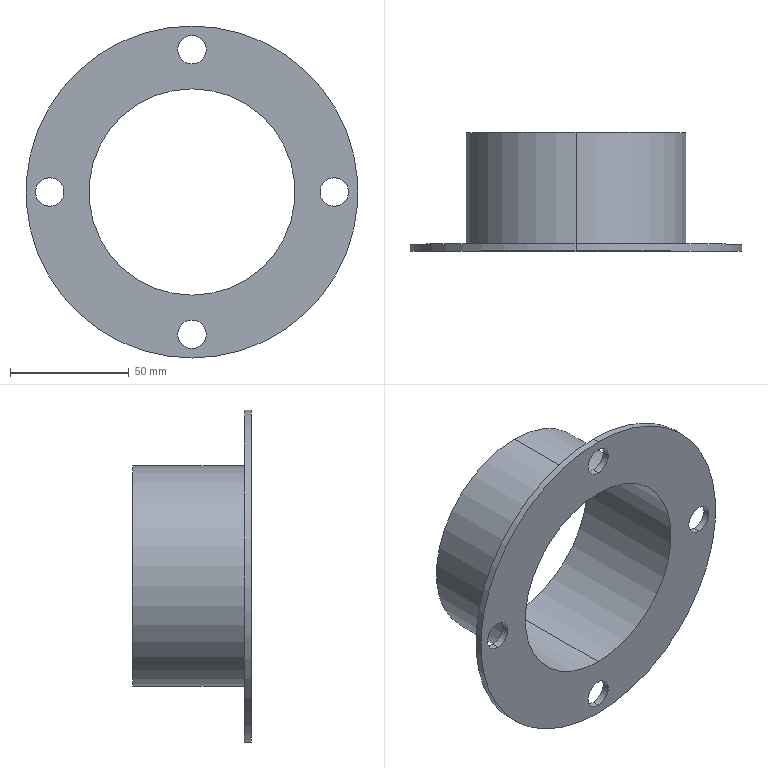Part | SolidWorks | features ICE 1, Revolution 1 | 1 solid | 17 faces | box 140 x 50 x 140 mm | volume 66857 mm3 | cylinder 14 | plane 3 | commonest cylinder face diameters 12 x8 87 x2 93 x2 140 x2
STEP:
#1=CARTESIAN_POINT('',(0.,0.,-66.));
#2=VERTEX_POINT('',#1);
#3=CARTESIAN_POINT('',(0.,0.,-54.));
#4=VERTEX_POINT('',#3);
#5=CARTESIAN_POINT('',(0.,0.,-60.));
#6=DIRECTION('',(0.,1.,0.));
#7=DIRECTION('',(0.,0.,1.));
#8=AXIS2_PLACEMENT_3D('',#5,#6,#7);
#9=CIRCLE('',#8,6.);
#10=EDGE_CURVE('',#2,#4,#9,.T.);
#11=ORIENTED_EDGE('',*,*,#10,.F.);
#12=CARTESIAN_POINT('',(0.,3.,-66.));
#13=VERTEX_POINT('',#12);
#14=CARTESIAN_POINT('',(0.,0.,-66.));
#15=DIRECTION('',(0.,1.,0.));
#16=VECTOR('',#15,1000.);
#17=LINE('',#14,#16);
#18=EDGE_CURVE('',#2,#13,#17,.T.);
#19=ORIENTED_EDGE('',*,*,#18,.T.);
#20=CARTESIAN_POINT('',(0.,3.,-54.));
#21=VERTEX_POINT('',#20);
#22=CARTESIAN_POINT('',(0.,3.,-60.));
#23=DIRECTION('',(0.,1.,0.));
#24=DIRECTION('',(0.,0.,1.));
#25=AXIS2_PLACEMENT_3D('',#22,#23,#24);
#26=CIRCLE('',#25,6.);
#27=EDGE_CURVE('',#13,#21,#26,.T.);
#28=ORIENTED_EDGE('',*,*,#27,.T.);
#29=CARTESIAN_POINT('',(0.,0.,-54.));
#30=DIRECTION('',(0.,1.,0.));
#31=VECTOR('',#30,1000.);
#32=LINE('',#29,#31);
#33=EDGE_CURVE('',#4,#21,#32,.T.);
#34=ORIENTED_EDGE('',*,*,#33,.F.);
#35=EDGE_LOOP('',(#11,#19,#28,#34));
#36=FACE_OUTER_BOUND('',#35,.T.);
#37=CARTESIAN_POINT('',(0.,0.,-60.));
#38=DIRECTION('',(0.,1.,0.));
#39=DIRECTION('',(0.,0.,1.));
#40=AXIS2_PLACEMENT_3D('',#37,#38,#39);
#41=CYLINDRICAL_SURFACE('',#40,6.);
#42=ADVANCED_FACE('',(#36),#41,.F.);
#43=CARTESIAN_POINT('',(60.,0.,-6.));
#44=VERTEX_POINT('',#43);
#45=CARTESIAN_POINT('',(60.,0.,6.));
#46=VERTEX_POINT('',#45);
#47=CARTESIAN_POINT('',(60.,0.,0.));
#48=DIRECTION('',(0.,1.,0.));
#49=DIRECTION('',(0.,0.,1.));
#50=AXIS2_PLACEMENT_3D('',#47,#48,#49);
#51=CIRCLE('',#50,6.);
#52=EDGE_CURVE('',#44,#46,#51,.T.);
#53=ORIENTED_EDGE('',*,*,#52,.F.);
#54=CARTESIAN_POINT('',(60.,3.,-6.));
#55=VERTEX_POINT('',#54);
#56=CARTESIAN_POINT('',(60.,0.,-6.));
#57=DIRECTION('',(0.,1.,0.));
#58=VECTOR('',#57,1000.);
#59=LINE('',#56,#58);
#60=EDGE_CURVE('',#44,#55,#59,.T.);
#61=ORIENTED_EDGE('',*,*,#60,.T.);
#62=CARTESIAN_POINT('',(60.,3.,6.));
#63=VERTEX_POINT('',#62);
#64=CARTESIAN_POINT('',(60.,3.,0.));
#65=DIRECTION('',(0.,1.,0.));
#66=DIRECTION('',(0.,0.,1.));
#67=AXIS2_PLACEMENT_3D('',#64,#65,#66);
#68=CIRCLE('',#67,6.);
#69=EDGE_CURVE('',#55,#63,#68,.T.);
#70=ORIENTED_EDGE('',*,*,#69,.T.);
#71=CARTESIAN_POINT('',(60.,0.,6.));
#72=DIRECTION('',(0.,1.,0.));
#73=VECTOR('',#72,1000.);
#74=LINE('',#71,#73);
#75=EDGE_CURVE('',#46,#63,#74,.T.);
#76=ORIENTED_EDGE('',*,*,#75,.F.);
#77=EDGE_LOOP('',(#53,#61,#70,#76));
#78=FACE_OUTER_BOUND('',#77,.T.);
#79=CARTESIAN_POINT('',(60.,0.,0.));
#80=DIRECTION('',(0.,1.,0.));
#81=DIRECTION('',(0.,0.,1.));
#82=AXIS2_PLACEMENT_3D('',#79,#80,#81);
#83=CYLINDRICAL_SURFACE('',#82,6.);
#84=ADVANCED_FACE('',(#78),#83,.F.);
#85=CARTESIAN_POINT('',(0.,0.,54.));
#86=VERTEX_POINT('',#85);
#87=CARTESIAN_POINT('',(0.,0.,66.));
#88=VERTEX_POINT('',#87);
#89=CARTESIAN_POINT('',(0.,0.,60.));
#90=DIRECTION('',(0.,1.,0.));
#91=DIRECTION('',(0.,0.,1.));
#92=AXIS2_PLACEMENT_3D('',#89,#90,#91);
#93=CIRCLE('',#92,6.);
#94=EDGE_CURVE('',#86,#88,#93,.T.);
#95=ORIENTED_EDGE('',*,*,#94,.F.);
#96=CARTESIAN_POINT('',(0.,3.,54.));
#97=VERTEX_POINT('',#96);
#98=CARTESIAN_POINT('',(0.,0.,54.));
#99=DIRECTION('',(0.,1.,0.));
#100=VECTOR('',#99,1000.);
#101=LINE('',#98,#100);
#102=EDGE_CURVE('',#86,#97,#101,.T.);
#103=ORIENTED_EDGE('',*,*,#102,.T.);
#104=CARTESIAN_POINT('',(0.,3.,66.));
#105=VERTEX_POINT('',#104);
#106=CARTESIAN_POINT('',(0.,3.,60.));
#107=DIRECTION('',(0.,1.,0.));
#108=DIRECTION('',(0.,0.,1.));
#109=AXIS2_PLACEMENT_3D('',#106,#107,#108);
#110=CIRCLE('',#109,6.);
#111=EDGE_CURVE('',#97,#105,#110,.T.);
#112=ORIENTED_EDGE('',*,*,#111,.T.);
#113=CARTESIAN_POINT('',(0.,0.,66.));
#114=DIRECTION('',(0.,1.,0.));
#115=VECTOR('',#114,1000.);
#116=LINE('',#113,#115);
#117=EDGE_CURVE('',#88,#105,#116,.T.);
#118=ORIENTED_EDGE('',*,*,#117,.F.);
#119=EDGE_LOOP('',(#95,#103,#112,#118));
#120=FACE_OUTER_BOUND('',#119,.T.);
#121=CARTESIAN_POINT('',(0.,0.,60.));
#122=DIRECTION('',(0.,1.,0.));
#123=DIRECTION('',(0.,0.,1.));
#124=AXIS2_PLACEMENT_3D('',#121,#122,#123);
#125=CYLINDRICAL_SURFACE('',#124,6.);
#126=ADVANCED_FACE('',(#120),#125,.F.);
#127=CARTESIAN_POINT('',(-60.,0.,-6.));
#128=VERTEX_POINT('',#127);
#129=CARTESIAN_POINT('',(-60.,0.,6.));
#130=VERTEX_POINT('',#129);
#131=CARTESIAN_POINT('',(-60.,0.,0.));
#132=DIRECTION('',(0.,1.,0.));
#133=DIRECTION('',(0.,0.,1.));
#134=AXIS2_PLACEMENT_3D('',#131,#132,#133);
#135=CIRCLE('',#134,6.);
#136=EDGE_CURVE('',#128,#130,#135,.T.);
#137=ORIENTED_EDGE('',*,*,#136,.F.);
#138=CARTESIAN_POINT('',(-60.,3.,-6.));
#139=VERTEX_POINT('',#138);
#140=CARTESIAN_POINT('',(-60.,0.,-6.));
#141=DIRECTION('',(0.,1.,0.));
#142=VECTOR('',#141,1000.);
#143=LINE('',#140,#142);
#144=EDGE_CURVE('',#128,#139,#143,.T.);
#145=ORIENTED_EDGE('',*,*,#144,.T.);
#146=CARTESIAN_POINT('',(-60.,3.,6.));
#147=VERTEX_POINT('',#146);
#148=CARTESIAN_POINT('',(-60.,3.,0.));
#149=DIRECTION('',(0.,1.,0.));
#150=DIRECTION('',(0.,0.,1.));
#151=AXIS2_PLACEMENT_3D('',#148,#149,#150);
#152=CIRCLE('',#151,6.);
#153=EDGE_CURVE('',#139,#147,#152,.T.);
#154=ORIENTED_EDGE('',*,*,#153,.T.);
#155=CARTESIAN_POINT('',(-60.,0.,6.));
#156=DIRECTION('',(0.,1.,0.));
#157=VECTOR('',#156,1000.);
#158=LINE('',#155,#157);
#159=EDGE_CURVE('',#130,#147,#158,.T.);
#160=ORIENTED_EDGE('',*,*,#159,.F.);
#161=EDGE_LOOP('',(#137,#145,#154,#160));
#162=FACE_OUTER_BOUND('',#161,.T.);
#163=CARTESIAN_POINT('',(-60.,0.,0.));
#164=DIRECTION('',(0.,1.,0.));
#165=DIRECTION('',(0.,0.,1.));
#166=AXIS2_PLACEMENT_3D('',#163,#164,#165);
#167=CYLINDRICAL_SURFACE('',#166,6.);
#168=ADVANCED_FACE('',(#162),#167,.F.);
#169=CARTESIAN_POINT('',(0.,50.,43.5));
#170=VERTEX_POINT('',#169);
#171=CARTESIAN_POINT('',(0.,50.,-43.5));
#172=VERTEX_POINT('',#171);
#173=CARTESIAN_POINT('',(0.,50.,0.));
#174=DIRECTION('',(0.,-1.,0.));
#175=DIRECTION('',(0.,0.,-1.));
#176=AXIS2_PLACEMENT_3D('',#173,#174,#175);
#177=CIRCLE('',#176,43.5);
#178=EDGE_CURVE('',#170,#172,#177,.T.);
#179=ORIENTED_EDGE('',*,*,#178,.F.);
#180=CARTESIAN_POINT('',(0.,0.,43.5));
#181=VERTEX_POINT('',#180);
#182=CARTESIAN_POINT('',(0.,0.,43.5));
#183=DIRECTION('',(0.,-1.,0.));
#184=VECTOR('',#183,1000.);
#185=LINE('',#182,#184);
#186=EDGE_CURVE('',#170,#181,#185,.T.);
#187=ORIENTED_EDGE('',*,*,#186,.T.);
#188=CARTESIAN_POINT('',(0.,0.,-43.5));
#189=VERTEX_POINT('',#188);
#190=CARTESIAN_POINT('',(0.,0.,0.));
#191=DIRECTION('',(0.,-1.,0.));
#192=DIRECTION('',(0.,0.,-1.));
#193=AXIS2_PLACEMENT_3D('',#190,#191,#192);
#194=CIRCLE('',#193,43.5);
#195=EDGE_CURVE('',#181,#189,#194,.T.);
#196=ORIENTED_EDGE('',*,*,#195,.T.);
#197=CARTESIAN_POINT('',(0.,0.,-43.5));
#198=DIRECTION('',(0.,-1.,0.));
#199=VECTOR('',#198,1000.);
#200=LINE('',#197,#199);
#201=EDGE_CURVE('',#172,#189,#200,.T.);
#202=ORIENTED_EDGE('',*,*,#201,.F.);
#203=EDGE_LOOP('',(#179,#187,#196,#202));
#204=FACE_OUTER_BOUND('',#203,.T.);
#205=CARTESIAN_POINT('',(0.,0.,0.));
#206=DIRECTION('',(0.,-1.,0.));
#207=DIRECTION('',(0.,0.,-1.));
#208=AXIS2_PLACEMENT_3D('',#205,#206,#207);
#209=CYLINDRICAL_SURFACE('',#208,43.5);
#210=ADVANCED_FACE('',(#204),#209,.F.);
#211=CARTESIAN_POINT('',(0.,3.,-70.));
#212=VERTEX_POINT('',#211);
#213=CARTESIAN_POINT('',(0.,3.,70.));
#214=VERTEX_POINT('',#213);
#215=CARTESIAN_POINT('',(0.,3.,0.));
#216=DIRECTION('',(0.,-1.,0.));
#217=DIRECTION('',(0.,0.,-1.));
#218=AXIS2_PLACEMENT_3D('',#215,#216,#217);
#219=CIRCLE('',#218,70.);
#220=EDGE_CURVE('',#212,#214,#219,.T.);
#221=ORIENTED_EDGE('',*,*,#220,.T.);
#222=CARTESIAN_POINT('',(0.,0.,70.));
#223=VERTEX_POINT('',#222);
#224=CARTESIAN_POINT('',(0.,0.,70.));
#225=DIRECTION('',(0.,-1.,0.));
#226=VECTOR('',#225,1000.);
#227=LINE('',#224,#226);
#228=EDGE_CURVE('',#214,#223,#227,.T.);
#229=ORIENTED_EDGE('',*,*,#228,.T.);
#230=CARTESIAN_POINT('',(0.,0.,-70.));
#231=VERTEX_POINT('',#230);
#232=CARTESIAN_POINT('',(0.,0.,0.));
#233=DIRECTION('',(0.,-1.,0.));
#234=DIRECTION('',(0.,0.,-1.));
#235=AXIS2_PLACEMENT_3D('',#232,#233,#234);
#236=CIRCLE('',#235,70.);
#237=EDGE_CURVE('',#231,#223,#236,.T.);
#238=ORIENTED_EDGE('',*,*,#237,.F.);
#239=CARTESIAN_POINT('',(0.,0.,-70.));
#240=DIRECTION('',(0.,-1.,0.));
#241=VECTOR('',#240,1000.);
#242=LINE('',#239,#241);
#243=EDGE_CURVE('',#212,#231,#242,.T.);
#244=ORIENTED_EDGE('',*,*,#243,.F.);
#245=EDGE_LOOP('',(#221,#229,#238,#244));
#246=FACE_OUTER_BOUND('',#245,.T.);
#247=CARTESIAN_POINT('',(0.,0.,0.));
#248=DIRECTION('',(0.,-1.,0.));
#249=DIRECTION('',(0.,0.,-1.));
#250=AXIS2_PLACEMENT_3D('',#247,#248,#249);
#251=CYLINDRICAL_SURFACE('',#250,70.);
#252=ADVANCED_FACE('',(#246),#251,.T.);
#253=CARTESIAN_POINT('',(0.,50.,-46.5));
#254=VERTEX_POINT('',#253);
#255=CARTESIAN_POINT('',(0.,50.,46.5));
#256=VERTEX_POINT('',#255);
#257=CARTESIAN_POINT('',(0.,50.,0.));
#258=DIRECTION('',(0.,-1.,0.));
#259=DIRECTION('',(0.,0.,-1.));
#260=AXIS2_PLACEMENT_3D('',#257,#258,#259);
#261=CIRCLE('',#260,46.5);
#262=EDGE_CURVE('',#254,#256,#261,.T.);
#263=ORIENTED_EDGE('',*,*,#262,.T.);
#264=CARTESIAN_POINT('',(0.,3.,46.5));
#265=VERTEX_POINT('',#264);
#266=CARTESIAN_POINT('',(0.,0.,46.5));
#267=DIRECTION('',(0.,-1.,0.));
#268=VECTOR('',#267,1000.);
#269=LINE('',#266,#268);
#270=EDGE_CURVE('',#256,#265,#269,.T.);
#271=ORIENTED_EDGE('',*,*,#270,.T.);
#272=CARTESIAN_POINT('',(0.,3.,-46.5));
#273=VERTEX_POINT('',#272);
#274=CARTESIAN_POINT('',(0.,3.,0.));
#275=DIRECTION('',(0.,-1.,0.));
#276=DIRECTION('',(0.,0.,-1.));
#277=AXIS2_PLACEMENT_3D('',#274,#275,#276);
#278=CIRCLE('',#277,46.5);
#279=EDGE_CURVE('',#273,#265,#278,.T.);
#280=ORIENTED_EDGE('',*,*,#279,.F.);
#281=CARTESIAN_POINT('',(0.,0.,-46.5));
#282=DIRECTION('',(0.,-1.,0.));
#283=VECTOR('',#282,1000.);
#284=LINE('',#281,#283);
#285=EDGE_CURVE('',#254,#273,#284,.T.);
#286=ORIENTED_EDGE('',*,*,#285,.F.);
#287=EDGE_LOOP('',(#263,#271,#280,#286));
#288=FACE_OUTER_BOUND('',#287,.T.);
#289=CARTESIAN_POINT('',(0.,0.,0.));
#290=DIRECTION('',(0.,-1.,0.));
#291=DIRECTION('',(0.,0.,-1.));
#292=AXIS2_PLACEMENT_3D('',#289,#290,#291);
#293=CYLINDRICAL_SURFACE('',#292,46.5);
#294=ADVANCED_FACE('',(#288),#293,.T.);
#295=CARTESIAN_POINT('',(0.,50.,0.));
#296=DIRECTION('',(0.,-1.,0.));
#297=DIRECTION('',(0.,0.,-1.));
#298=AXIS2_PLACEMENT_3D('',#295,#296,#297);
#299=CIRCLE('',#298,43.5);
#300=EDGE_CURVE('',#172,#170,#299,.T.);
#301=ORIENTED_EDGE('',*,*,#300,.T.);
#302=ORIENTED_EDGE('',*,*,#178,.T.);
#303=EDGE_LOOP('',(#301,#302));
#304=FACE_BOUND('',#303,.T.);
#305=ORIENTED_EDGE('',*,*,#262,.F.);
#306=CARTESIAN_POINT('',(0.,50.,0.));
#307=DIRECTION('',(0.,-1.,0.));
#308=DIRECTION('',(0.,0.,-1.));
#309=AXIS2_PLACEMENT_3D('',#306,#307,#308);
#310=CIRCLE('',#309,46.5);
#311=EDGE_CURVE('',#256,#254,#310,.T.);
#312=ORIENTED_EDGE('',*,*,#311,.F.);
#313=EDGE_LOOP('',(#305,#312));
#314=FACE_OUTER_BOUND('',#313,.T.);
#315=CARTESIAN_POINT('',(43.5,50.,0.));
#316=DIRECTION('',(0.,1.,0.));
#317=DIRECTION('',(0.,0.,1.));
#318=AXIS2_PLACEMENT_3D('',#315,#316,#317);
#319=PLANE('',#318);
#320=ADVANCED_FACE('',(#304,#314),#319,.T.);
#321=ORIENTED_EDGE('',*,*,#270,.F.);
#322=ORIENTED_EDGE('',*,*,#311,.T.);
#323=ORIENTED_EDGE('',*,*,#285,.T.);
#324=CARTESIAN_POINT('',(0.,3.,0.));
#325=DIRECTION('',(0.,-1.,0.));
#326=DIRECTION('',(0.,0.,-1.));
#327=AXIS2_PLACEMENT_3D('',#324,#325,#326);
#328=CIRCLE('',#327,46.5);
#329=EDGE_CURVE('',#265,#273,#328,.T.);
#330=ORIENTED_EDGE('',*,*,#329,.F.);
#331=EDGE_LOOP('',(#321,#322,#323,#330));
#332=FACE_OUTER_BOUND('',#331,.T.);
#333=CARTESIAN_POINT('',(0.,0.,0.));
#334=DIRECTION('',(0.,-1.,0.));
#335=DIRECTION('',(0.,0.,-1.));
#336=AXIS2_PLACEMENT_3D('',#333,#334,#335);
#337=CYLINDRICAL_SURFACE('',#336,46.5);
#338=ADVANCED_FACE('',(#332),#337,.T.);
#339=CARTESIAN_POINT('',(0.,3.,-60.));
#340=DIRECTION('',(0.,1.,0.));
#341=DIRECTION('',(0.,0.,1.));
#342=AXIS2_PLACEMENT_3D('',#339,#340,#341);
#343=CIRCLE('',#342,6.);
#344=EDGE_CURVE('',#21,#13,#343,.T.);
#345=ORIENTED_EDGE('',*,*,#344,.F.);
#346=ORIENTED_EDGE('',*,*,#27,.F.);
#347=EDGE_LOOP('',(#345,#346));
#348=FACE_BOUND('',#347,.T.);
#349=CARTESIAN_POINT('',(60.,3.,0.));
#350=DIRECTION('',(0.,1.,0.));
#351=DIRECTION('',(0.,0.,1.));
#352=AXIS2_PLACEMENT_3D('',#349,#350,#351);
#353=CIRCLE('',#352,6.);
#354=EDGE_CURVE('',#63,#55,#353,.T.);
#355=ORIENTED_EDGE('',*,*,#354,.F.);
#356=ORIENTED_EDGE('',*,*,#69,.F.);
#357=EDGE_LOOP('',(#355,#356));
#358=FACE_BOUND('',#357,.T.);
#359=CARTESIAN_POINT('',(0.,3.,60.));
#360=DIRECTION('',(0.,1.,0.));
#361=DIRECTION('',(0.,0.,1.));
#362=AXIS2_PLACEMENT_3D('',#359,#360,#361);
#363=CIRCLE('',#362,6.);
#364=EDGE_CURVE('',#105,#97,#363,.T.);
#365=ORIENTED_EDGE('',*,*,#364,.F.);
#366=ORIENTED_EDGE('',*,*,#111,.F.);
#367=EDGE_LOOP('',(#365,#366));
#368=FACE_BOUND('',#367,.T.);
#369=CARTESIAN_POINT('',(-60.,3.,0.));
#370=DIRECTION('',(0.,1.,0.));
#371=DIRECTION('',(0.,0.,1.));
#372=AXIS2_PLACEMENT_3D('',#369,#370,#371);
#373=CIRCLE('',#372,6.);
#374=EDGE_CURVE('',#147,#139,#373,.T.);
#375=ORIENTED_EDGE('',*,*,#374,.F.);
#376=ORIENTED_EDGE('',*,*,#153,.F.);
#377=EDGE_LOOP('',(#375,#376));
#378=FACE_BOUND('',#377,.T.);
#379=ORIENTED_EDGE('',*,*,#279,.T.);
#380=ORIENTED_EDGE('',*,*,#329,.T.);
#381=EDGE_LOOP('',(#379,#380));
#382=FACE_BOUND('',#381,.T.);
#383=ORIENTED_EDGE('',*,*,#220,.F.);
#384=CARTESIAN_POINT('',(0.,3.,0.));
#385=DIRECTION('',(0.,-1.,0.));
#386=DIRECTION('',(0.,0.,-1.));
#387=AXIS2_PLACEMENT_3D('',#384,#385,#386);
#388=CIRCLE('',#387,70.);
#389=EDGE_CURVE('',#214,#212,#388,.T.);
#390=ORIENTED_EDGE('',*,*,#389,.F.);
#391=EDGE_LOOP('',(#383,#390));
#392=FACE_OUTER_BOUND('',#391,.T.);
#393=CARTESIAN_POINT('',(46.5,3.,0.));
#394=DIRECTION('',(0.,1.,0.));
#395=DIRECTION('',(0.,0.,1.));
#396=AXIS2_PLACEMENT_3D('',#393,#394,#395);
#397=PLANE('',#396);
#398=ADVANCED_FACE('',(#348,#358,#368,#378,#382,#392),#397,.T.);
#399=ORIENTED_EDGE('',*,*,#228,.F.);
#400=ORIENTED_EDGE('',*,*,#389,.T.);
#401=ORIENTED_EDGE('',*,*,#243,.T.);
#402=CARTESIAN_POINT('',(0.,0.,0.));
#403=DIRECTION('',(0.,-1.,0.));
#404=DIRECTION('',(0.,0.,-1.));
#405=AXIS2_PLACEMENT_3D('',#402,#403,#404);
#406=CIRCLE('',#405,70.);
#407=EDGE_CURVE('',#223,#231,#406,.T.);
#408=ORIENTED_EDGE('',*,*,#407,.F.);
#409=EDGE_LOOP('',(#399,#400,#401,#408));
#410=FACE_OUTER_BOUND('',#409,.T.);
#411=CARTESIAN_POINT('',(0.,0.,0.));
#412=DIRECTION('',(0.,-1.,0.));
#413=DIRECTION('',(0.,0.,-1.));
#414=AXIS2_PLACEMENT_3D('',#411,#412,#413);
#415=CYLINDRICAL_SURFACE('',#414,70.);
#416=ADVANCED_FACE('',(#410),#415,.T.);
#417=CARTESIAN_POINT('',(0.,0.,-60.));
#418=DIRECTION('',(0.,1.,0.));
#419=DIRECTION('',(0.,0.,1.));
#420=AXIS2_PLACEMENT_3D('',#417,#418,#419);
#421=CIRCLE('',#420,6.);
#422=EDGE_CURVE('',#4,#2,#421,.T.);
#423=ORIENTED_EDGE('',*,*,#422,.T.);
#424=ORIENTED_EDGE('',*,*,#10,.T.);
#425=EDGE_LOOP('',(#423,#424));
#426=FACE_BOUND('',#425,.T.);
#427=CARTESIAN_POINT('',(60.,0.,0.));
#428=DIRECTION('',(0.,1.,0.));
#429=DIRECTION('',(0.,0.,1.));
#430=AXIS2_PLACEMENT_3D('',#427,#428,#429);
#431=CIRCLE('',#430,6.);
#432=EDGE_CURVE('',#46,#44,#431,.T.);
#433=ORIENTED_EDGE('',*,*,#432,.T.);
#434=ORIENTED_EDGE('',*,*,#52,.T.);
#435=EDGE_LOOP('',(#433,#434));
#436=FACE_BOUND('',#435,.T.);
#437=CARTESIAN_POINT('',(0.,0.,60.));
#438=DIRECTION('',(0.,1.,0.));
#439=DIRECTION('',(0.,0.,1.));
#440=AXIS2_PLACEMENT_3D('',#437,#438,#439);
#441=CIRCLE('',#440,6.);
#442=EDGE_CURVE('',#88,#86,#441,.T.);
#443=ORIENTED_EDGE('',*,*,#442,.T.);
#444=ORIENTED_EDGE('',*,*,#94,.T.);
#445=EDGE_LOOP('',(#443,#444));
#446=FACE_BOUND('',#445,.T.);
#447=CARTESIAN_POINT('',(-60.,0.,0.));
#448=DIRECTION('',(0.,1.,0.));
#449=DIRECTION('',(0.,0.,1.));
#450=AXIS2_PLACEMENT_3D('',#447,#448,#449);
#451=CIRCLE('',#450,6.);
#452=EDGE_CURVE('',#130,#128,#451,.T.);
#453=ORIENTED_EDGE('',*,*,#452,.T.);
#454=ORIENTED_EDGE('',*,*,#136,.T.);
#455=EDGE_LOOP('',(#453,#454));
#456=FACE_BOUND('',#455,.T.);
#457=ORIENTED_EDGE('',*,*,#237,.T.);
#458=ORIENTED_EDGE('',*,*,#407,.T.);
#459=EDGE_LOOP('',(#457,#458));
#460=FACE_OUTER_BOUND('',#459,.T.);
#461=CARTESIAN_POINT('',(0.,0.,0.));
#462=DIRECTION('',(0.,-1.,0.));
#463=DIRECTION('',(0.,0.,-1.));
#464=AXIS2_PLACEMENT_3D('',#461,#462,#463);
#465=CIRCLE('',#464,43.5);
#466=EDGE_CURVE('',#189,#181,#465,.T.);
#467=ORIENTED_EDGE('',*,*,#466,.F.);
#468=ORIENTED_EDGE('',*,*,#195,.F.);
#469=EDGE_LOOP('',(#467,#468));
#470=FACE_BOUND('',#469,.T.);
#471=CARTESIAN_POINT('',(43.5,0.,0.));
#472=DIRECTION('',(0.,-1.,0.));
#473=DIRECTION('',(0.,0.,-1.));
#474=AXIS2_PLACEMENT_3D('',#471,#472,#473);
#475=PLANE('',#474);
#476=ADVANCED_FACE('',(#426,#436,#446,#456,#460,#470),#475,.T.);
#477=ORIENTED_EDGE('',*,*,#186,.F.);
#478=ORIENTED_EDGE('',*,*,#300,.F.);
#479=ORIENTED_EDGE('',*,*,#201,.T.);
#480=ORIENTED_EDGE('',*,*,#466,.T.);
#481=EDGE_LOOP('',(#477,#478,#479,#480));
#482=FACE_OUTER_BOUND('',#481,.T.);
#483=CARTESIAN_POINT('',(0.,0.,0.));
#484=DIRECTION('',(0.,-1.,0.));
#485=DIRECTION('',(0.,0.,-1.));
#486=AXIS2_PLACEMENT_3D('',#483,#484,#485);
#487=CYLINDRICAL_SURFACE('',#486,43.5);
#488=ADVANCED_FACE('',(#482),#487,.F.);
#489=ORIENTED_EDGE('',*,*,#144,.F.);
#490=ORIENTED_EDGE('',*,*,#452,.F.);
#491=ORIENTED_EDGE('',*,*,#159,.T.);
#492=ORIENTED_EDGE('',*,*,#374,.T.);
#493=EDGE_LOOP('',(#489,#490,#491,#492));
#494=FACE_OUTER_BOUND('',#493,.T.);
#495=CARTESIAN_POINT('',(-60.,0.,0.));
#496=DIRECTION('',(0.,1.,0.));
#497=DIRECTION('',(0.,0.,1.));
#498=AXIS2_PLACEMENT_3D('',#495,#496,#497);
#499=CYLINDRICAL_SURFACE('',#498,6.);
#500=ADVANCED_FACE('',(#494),#499,.F.);
#501=ORIENTED_EDGE('',*,*,#102,.F.);
#502=ORIENTED_EDGE('',*,*,#442,.F.);
#503=ORIENTED_EDGE('',*,*,#117,.T.);
#504=ORIENTED_EDGE('',*,*,#364,.T.);
#505=EDGE_LOOP('',(#501,#502,#503,#504));
#506=FACE_OUTER_BOUND('',#505,.T.);
#507=CARTESIAN_POINT('',(0.,0.,60.));
#508=DIRECTION('',(0.,1.,0.));
#509=DIRECTION('',(0.,0.,1.));
#510=AXIS2_PLACEMENT_3D('',#507,#508,#509);
#511=CYLINDRICAL_SURFACE('',#510,6.);
#512=ADVANCED_FACE('',(#506),#511,.F.);
#513=ORIENTED_EDGE('',*,*,#60,.F.);
#514=ORIENTED_EDGE('',*,*,#432,.F.);
#515=ORIENTED_EDGE('',*,*,#75,.T.);
#516=ORIENTED_EDGE('',*,*,#354,.T.);
#517=EDGE_LOOP('',(#513,#514,#515,#516));
#518=FACE_OUTER_BOUND('',#517,.T.);
#519=CARTESIAN_POINT('',(60.,0.,0.));
#520=DIRECTION('',(0.,1.,0.));
#521=DIRECTION('',(0.,0.,1.));
#522=AXIS2_PLACEMENT_3D('',#519,#520,#521);
#523=CYLINDRICAL_SURFACE('',#522,6.);
#524=ADVANCED_FACE('',(#518),#523,.F.);
#525=ORIENTED_EDGE('',*,*,#18,.F.);
#526=ORIENTED_EDGE('',*,*,#422,.F.);
#527=ORIENTED_EDGE('',*,*,#33,.T.);
#528=ORIENTED_EDGE('',*,*,#344,.T.);
#529=EDGE_LOOP('',(#525,#526,#527,#528));
#530=FACE_OUTER_BOUND('',#529,.T.);
#531=CARTESIAN_POINT('',(0.,0.,-60.));
#532=DIRECTION('',(0.,1.,0.));
#533=DIRECTION('',(0.,0.,1.));
#534=AXIS2_PLACEMENT_3D('',#531,#532,#533);
#535=CYLINDRICAL_SURFACE('',#534,6.);
#536=ADVANCED_FACE('',(#530),#535,.F.);
#537=CLOSED_SHELL('',(#42,#84,#126,#168,#210,#252,#294,#320,#338,#398,#416,#476,#488,#500,#512,#524,#536));
#538=MANIFOLD_SOLID_BREP('',#537);
#539=CARTESIAN_POINT('',(0.,0.,0.));
#540=DIRECTION('',(0.,0.,1.));
#541=DIRECTION('',(1.,0.,0.));
#542=AXIS2_PLACEMENT_3D('',#539,#540,#541);
#543=(LENGTH_UNIT()NAMED_UNIT(*)SI_UNIT(.MILLI.,.METRE.));
#544=UNCERTAINTY_MEASURE_WITH_UNIT(LENGTH_MEASURE(0.00001),#543,'','');
#545=(NAMED_UNIT(*)PLANE_ANGLE_UNIT()SI_UNIT($,.RADIAN.));
#546=(NAMED_UNIT(*)SI_UNIT($,.STERADIAN.)SOLID_ANGLE_UNIT());
#547=(GEOMETRIC_REPRESENTATION_CONTEXT(3)GLOBAL_UNCERTAINTY_ASSIGNED_CONTEXT((#544))GLOBAL_UNIT_ASSIGNED_CONTEXT((#543,#545,#546))REPRESENTATION_CONTEXT('',''));
#548=ADVANCED_BREP_SHAPE_REPRESENTATION('',(#538,#542),#547);